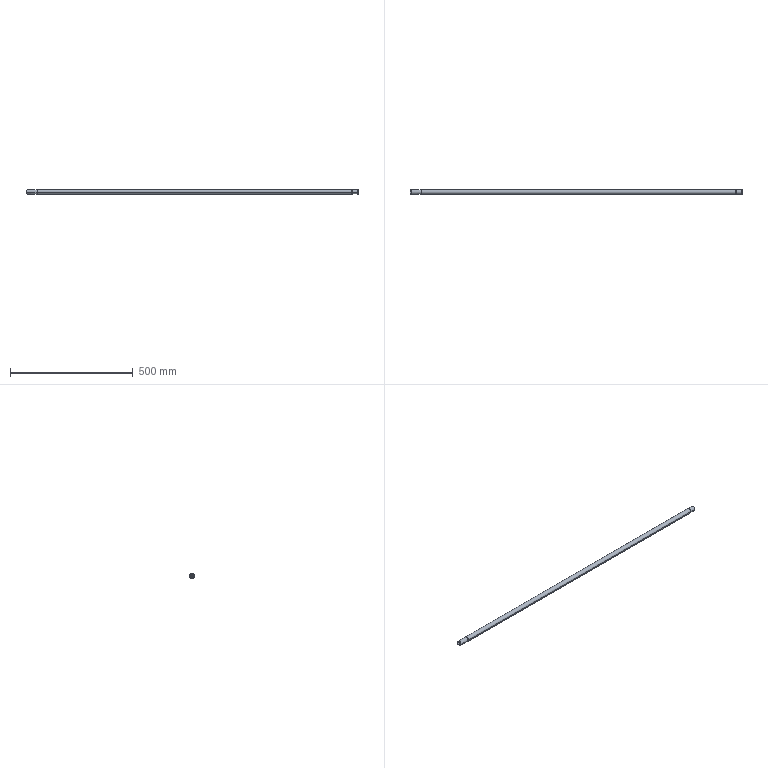Part | STEP file | DCV-000-009 | 1 solid | 34 faces | box 1354 x 20 x 20 mm | volume 419638 mm3 | cylinder 14 | cone 10 | plane 10 | commonest cylinder face diameters 20 x6 10.106 x4 19 x4